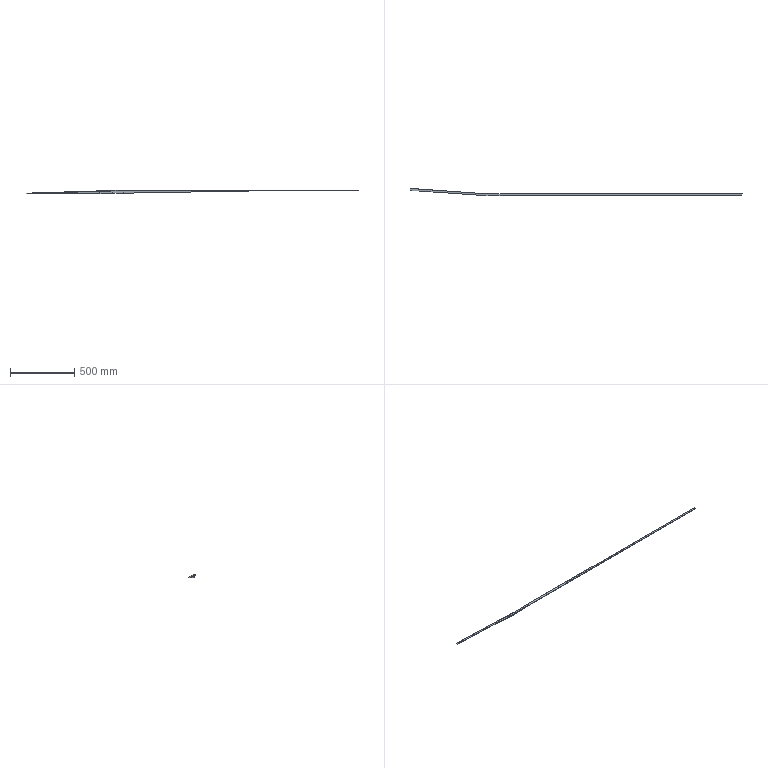Part | SolidWorks | features BaseBody 1 | 1 solid | 24 faces | box 2576 x 55.445 x 25.01 mm | volume 179602 mm3 | plane 24
STEP:
#1=CARTESIAN_POINT('',(1223.741,60.698,-2.475));
#2=VERTEX_POINT('',#1);
#3=CARTESIAN_POINT('',(180.528,60.974,-20.535));
#4=VERTEX_POINT('',#3);
#5=CARTESIAN_POINT('',(1223.741,60.698,-2.475));
#6=DIRECTION('',(-0.9999,0.0002647,-0.01731));
#7=VECTOR('',#6,1000.);
#8=LINE('',#5,#7);
#9=EDGE_CURVE('',#2,#4,#8,.T.);
#10=ORIENTED_EDGE('',*,*,#9,.F.);
#11=CARTESIAN_POINT('',(180.52,60.706,-2.934));
#12=VERTEX_POINT('',#11);
#13=CARTESIAN_POINT('',(180.52,60.706,-2.934));
#14=DIRECTION('',(1.,-0.000007674,0.0004396));
#15=VECTOR('',#14,1000.);
#16=LINE('',#13,#15);
#17=EDGE_CURVE('',#12,#2,#16,.T.);
#18=ORIENTED_EDGE('',*,*,#17,.F.);
#19=CARTESIAN_POINT('',(180.528,60.974,-20.535));
#20=DIRECTION('',(-0.0004397,-0.01523,0.9999));
#21=VECTOR('',#20,1000.);
#22=LINE('',#19,#21);
#23=EDGE_CURVE('',#4,#12,#22,.T.);
#24=ORIENTED_EDGE('',*,*,#23,.F.);
#25=EDGE_LOOP('',(#10,#18,#24));
#26=FACE_OUTER_BOUND('',#25,.T.);
#27=CARTESIAN_POINT('',(174.261,60.976,-20.643));
#28=DIRECTION('',(0.000000977,0.9999,0.01523));
#29=DIRECTION('',(0.,-0.01523,0.9999));
#30=AXIS2_PLACEMENT_3D('',#27,#28,#29);
#31=PLANE('',#30);
#32=ADVANCED_FACE('',(#26),#31,.F.);
#33=CARTESIAN_POINT('',(97.321,60.705,-2.934));
#34=VERTEX_POINT('',#33);
#35=CARTESIAN_POINT('',(180.52,60.706,-2.934));
#36=DIRECTION('',(-1.,-0.00001057,-0.000006272));
#37=VECTOR('',#36,1000.);
#38=LINE('',#35,#37);
#39=EDGE_CURVE('',#12,#34,#38,.T.);
#40=ORIENTED_EDGE('',*,*,#39,.T.);
#41=CARTESIAN_POINT('',(97.601,60.973,-20.536));
#42=VERTEX_POINT('',#41);
#43=CARTESIAN_POINT('',(97.321,60.705,-2.934));
#44=DIRECTION('',(0.01588,0.01523,-0.9998));
#45=VECTOR('',#44,1000.);
#46=LINE('',#43,#45);
#47=EDGE_CURVE('',#34,#42,#46,.T.);
#48=ORIENTED_EDGE('',*,*,#47,.T.);
#49=CARTESIAN_POINT('',(97.601,60.973,-20.536));
#50=DIRECTION('',(1.,0.00001057,0.000006272));
#51=VECTOR('',#50,1000.);
#52=LINE('',#49,#51);
#53=EDGE_CURVE('',#42,#4,#52,.T.);
#54=ORIENTED_EDGE('',*,*,#53,.T.);
#55=ORIENTED_EDGE('',*,*,#23,.T.);
#56=EDGE_LOOP('',(#40,#48,#54,#55));
#57=FACE_OUTER_BOUND('',#56,.T.);
#58=CARTESIAN_POINT('',(96.822,60.703,-2.828));
#59=DIRECTION('',(0.00001066,-0.9999,-0.01523));
#60=DIRECTION('',(0.,0.01523,-0.9999));
#61=AXIS2_PLACEMENT_3D('',#58,#59,#60);
#62=PLANE('',#61);
#63=ADVANCED_FACE('',(#57),#62,.T.);
#64=ORIENTED_EDGE('',*,*,#9,.T.);
#65=CARTESIAN_POINT('',(180.528,64.174,-20.486));
#66=VERTEX_POINT('',#65);
#67=CARTESIAN_POINT('',(180.528,60.954,-20.535));
#68=DIRECTION('',(0.,-0.9999,-0.01523));
#69=VECTOR('',#68,1000.);
#70=LINE('',#67,#69);
#71=EDGE_CURVE('',#66,#4,#70,.T.);
#72=ORIENTED_EDGE('',*,*,#71,.F.);
#73=CARTESIAN_POINT('',(1223.741,63.897,-2.427));
#74=VERTEX_POINT('',#73);
#75=CARTESIAN_POINT('',(1223.741,63.897,-2.427));
#76=DIRECTION('',(-0.9999,0.0002647,-0.01731));
#77=VECTOR('',#76,1000.);
#78=LINE('',#75,#77);
#79=EDGE_CURVE('',#74,#66,#78,.T.);
#80=ORIENTED_EDGE('',*,*,#79,.F.);
#81=CARTESIAN_POINT('',(1223.741,63.897,-2.427));
#82=DIRECTION('',(0.,0.9999,0.01523));
#83=VECTOR('',#82,1000.);
#84=LINE('',#81,#83);
#85=EDGE_CURVE('',#2,#74,#84,.T.);
#86=ORIENTED_EDGE('',*,*,#85,.F.);
#87=EDGE_LOOP('',(#64,#72,#80,#86));
#88=FACE_OUTER_BOUND('',#87,.T.);
#89=CARTESIAN_POINT('',(174.269,60.677,-20.648));
#90=DIRECTION('',(-0.01731,-0.01523,0.9997));
#91=DIRECTION('',(0.9999,0.,0.01731));
#92=AXIS2_PLACEMENT_3D('',#89,#90,#91);
#93=PLANE('',#92);
#94=ADVANCED_FACE('',(#88),#93,.F.);
#95=ORIENTED_EDGE('',*,*,#17,.T.);
#96=ORIENTED_EDGE('',*,*,#85,.T.);
#97=CARTESIAN_POINT('',(2000.001,63.891,-2.085));
#98=VERTEX_POINT('',#97);
#99=CARTESIAN_POINT('',(2000.001,63.891,-2.085));
#100=DIRECTION('',(-1.,0.000007674,-0.0004396));
#101=VECTOR('',#100,1000.);
#102=LINE('',#99,#101);
#103=EDGE_CURVE('',#98,#74,#102,.T.);
#104=ORIENTED_EDGE('',*,*,#103,.F.);
#105=CARTESIAN_POINT('',(2000.001,48.891,-2.314));
#106=VERTEX_POINT('',#105);
#107=CARTESIAN_POINT('',(2000.001,48.891,-2.314));
#108=DIRECTION('',(0.000000977,0.9999,0.01523));
#109=VECTOR('',#108,1000.);
#110=LINE('',#107,#109);
#111=EDGE_CURVE('',#106,#98,#110,.T.);
#112=ORIENTED_EDGE('',*,*,#111,.F.);
#113=CARTESIAN_POINT('',(180.52,48.905,-3.114));
#114=VERTEX_POINT('',#113);
#115=CARTESIAN_POINT('',(180.52,48.905,-3.114));
#116=DIRECTION('',(1.,-0.000007674,0.0004396));
#117=VECTOR('',#116,1000.);
#118=LINE('',#115,#117);
#119=EDGE_CURVE('',#114,#106,#118,.T.);
#120=ORIENTED_EDGE('',*,*,#119,.F.);
#121=CARTESIAN_POINT('',(180.52,48.833,-3.115));
#122=DIRECTION('',(0.,-0.9999,-0.01523));
#123=VECTOR('',#122,1000.);
#124=LINE('',#121,#123);
#125=EDGE_CURVE('',#12,#114,#124,.T.);
#126=ORIENTED_EDGE('',*,*,#125,.F.);
#127=EDGE_LOOP('',(#95,#96,#104,#112,#120,#126));
#128=FACE_OUTER_BOUND('',#127,.T.);
#129=CARTESIAN_POINT('',(180.52,63.904,-2.885));
#130=DIRECTION('',(-0.0004397,-0.01523,0.9999));
#131=DIRECTION('',(0.,-0.9999,-0.01523));
#132=AXIS2_PLACEMENT_3D('',#129,#130,#131);
#133=PLANE('',#132);
#134=ADVANCED_FACE('',(#128),#133,.F.);
#135=CARTESIAN_POINT('',(-2.947,60.757,-6.119));
#136=VERTEX_POINT('',#135);
#137=CARTESIAN_POINT('',(-2.947,60.757,-6.119));
#138=DIRECTION('',(0.9995,-0.0005189,0.03175));
#139=VECTOR('',#138,1000.);
#140=LINE('',#137,#139);
#141=EDGE_CURVE('',#136,#34,#140,.T.);
#142=ORIENTED_EDGE('',*,*,#141,.F.);
#143=CARTESIAN_POINT('',(-2.388,61.025,-23.712));
#144=VERTEX_POINT('',#143);
#145=CARTESIAN_POINT('',(-2.388,61.025,-23.712));
#146=DIRECTION('',(-0.03175,-0.01522,0.9994));
#147=VECTOR('',#146,1000.);
#148=LINE('',#145,#147);
#149=EDGE_CURVE('',#144,#136,#148,.T.);
#150=ORIENTED_EDGE('',*,*,#149,.F.);
#151=CARTESIAN_POINT('',(97.601,60.973,-20.536));
#152=DIRECTION('',(-0.9995,0.0005189,-0.03175));
#153=VECTOR('',#152,1000.);
#154=LINE('',#151,#153);
#155=EDGE_CURVE('',#42,#144,#154,.T.);
#156=ORIENTED_EDGE('',*,*,#155,.F.);
#157=ORIENTED_EDGE('',*,*,#47,.F.);
#158=EDGE_LOOP('',(#142,#150,#156,#157));
#159=FACE_OUTER_BOUND('',#158,.T.);
#160=CARTESIAN_POINT('',(-3.55,61.027,-23.836));
#161=DIRECTION('',(0.00003526,0.9999,0.01523));
#162=DIRECTION('',(0.,-0.01523,0.9999));
#163=AXIS2_PLACEMENT_3D('',#160,#161,#162);
#164=PLANE('',#163);
#165=ADVANCED_FACE('',(#159),#164,.F.);
#166=CARTESIAN_POINT('',(97.321,48.904,-3.114));
#167=VERTEX_POINT('',#166);
#168=CARTESIAN_POINT('',(180.52,48.905,-3.114));
#169=DIRECTION('',(-1.,-0.00001057,-0.000006272));
#170=VECTOR('',#169,1000.);
#171=LINE('',#168,#170);
#172=EDGE_CURVE('',#114,#167,#171,.T.);
#173=ORIENTED_EDGE('',*,*,#172,.T.);
#174=CARTESIAN_POINT('',(97.321,48.904,-3.114));
#175=DIRECTION('',(0.00001231,0.9999,0.01523));
#176=VECTOR('',#175,1000.);
#177=LINE('',#174,#176);
#178=EDGE_CURVE('',#167,#34,#177,.T.);
#179=ORIENTED_EDGE('',*,*,#178,.T.);
#180=ORIENTED_EDGE('',*,*,#39,.F.);
#181=ORIENTED_EDGE('',*,*,#125,.T.);
#182=EDGE_LOOP('',(#173,#179,#180,#181));
#183=FACE_OUTER_BOUND('',#182,.T.);
#184=CARTESIAN_POINT('',(96.822,48.833,-3.115));
#185=DIRECTION('',(0.00000611,0.01523,-0.9999));
#186=DIRECTION('',(0.,0.9999,0.01523));
#187=AXIS2_PLACEMENT_3D('',#184,#185,#186);
#188=PLANE('',#187);
#189=ADVANCED_FACE('',(#183),#188,.T.);
#190=ORIENTED_EDGE('',*,*,#53,.F.);
#191=CARTESIAN_POINT('',(97.601,64.173,-20.487));
#192=VERTEX_POINT('',#191);
#193=CARTESIAN_POINT('',(97.601,60.973,-20.536));
#194=DIRECTION('',(0.00001231,0.9999,0.01523));
#195=VECTOR('',#194,1000.);
#196=LINE('',#193,#195);
#197=EDGE_CURVE('',#42,#192,#196,.T.);
#198=ORIENTED_EDGE('',*,*,#197,.T.);
#199=CARTESIAN_POINT('',(97.601,64.173,-20.487));
#200=DIRECTION('',(1.,0.00001057,0.000006272));
#201=VECTOR('',#200,1000.);
#202=LINE('',#199,#201);
#203=EDGE_CURVE('',#192,#66,#202,.T.);
#204=ORIENTED_EDGE('',*,*,#203,.T.);
#205=ORIENTED_EDGE('',*,*,#71,.T.);
#206=EDGE_LOOP('',(#190,#198,#204,#205));
#207=FACE_OUTER_BOUND('',#206,.T.);
#208=CARTESIAN_POINT('',(97.103,60.954,-20.536));
#209=DIRECTION('',(0.00000611,0.01523,-0.9999));
#210=DIRECTION('',(0.,0.9999,0.01523));
#211=AXIS2_PLACEMENT_3D('',#208,#209,#210);
#212=PLANE('',#211);
#213=ADVANCED_FACE('',(#207),#212,.T.);
#214=ORIENTED_EDGE('',*,*,#79,.T.);
#215=CARTESIAN_POINT('',(180.519,63.857,0.3145));
#216=VERTEX_POINT('',#215);
#217=CARTESIAN_POINT('',(180.519,63.857,0.3145));
#218=DIRECTION('',(0.0004397,0.01523,-0.9999));
#219=VECTOR('',#218,1000.);
#220=LINE('',#217,#219);
#221=EDGE_CURVE('',#216,#66,#220,.T.);
#222=ORIENTED_EDGE('',*,*,#221,.F.);
#223=CARTESIAN_POINT('',(2000.,63.843,1.114));
#224=VERTEX_POINT('',#223);
#225=CARTESIAN_POINT('',(2000.,63.843,1.114));
#226=DIRECTION('',(-1.,0.000007674,-0.0004396));
#227=VECTOR('',#226,1000.);
#228=LINE('',#225,#227);
#229=EDGE_CURVE('',#224,#216,#228,.T.);
#230=ORIENTED_EDGE('',*,*,#229,.F.);
#231=CARTESIAN_POINT('',(2000.001,63.891,-2.085));
#232=DIRECTION('',(-0.0004397,-0.01523,0.9999));
#233=VECTOR('',#232,1000.);
#234=LINE('',#231,#233);
#235=EDGE_CURVE('',#98,#224,#234,.T.);
#236=ORIENTED_EDGE('',*,*,#235,.F.);
#237=ORIENTED_EDGE('',*,*,#103,.T.);
#238=EDGE_LOOP('',(#214,#222,#230,#236,#237));
#239=FACE_OUTER_BOUND('',#238,.T.);
#240=CARTESIAN_POINT('',(180.519,63.844,1.114));
#241=DIRECTION('',(-0.000000977,-0.9999,-0.01523));
#242=DIRECTION('',(0.,0.01523,-0.9999));
#243=AXIS2_PLACEMENT_3D('',#240,#241,#242);
#244=PLANE('',#243);
#245=ADVANCED_FACE('',(#239),#244,.F.);
#246=CARTESIAN_POINT('',(2000.,48.842,0.8859));
#247=VERTEX_POINT('',#246);
#248=CARTESIAN_POINT('',(2000.,63.843,1.114));
#249=DIRECTION('',(-0.000000977,-0.9999,-0.01523));
#250=VECTOR('',#249,1000.);
#251=LINE('',#248,#250);
#252=EDGE_CURVE('',#224,#247,#251,.T.);
#253=ORIENTED_EDGE('',*,*,#252,.T.);
#254=CARTESIAN_POINT('',(2000.,48.842,0.8859));
#255=DIRECTION('',(0.0004397,0.01523,-0.9999));
#256=VECTOR('',#255,1000.);
#257=LINE('',#254,#256);
#258=EDGE_CURVE('',#247,#106,#257,.T.);
#259=ORIENTED_EDGE('',*,*,#258,.T.);
#260=ORIENTED_EDGE('',*,*,#111,.T.);
#261=ORIENTED_EDGE('',*,*,#235,.T.);
#262=EDGE_LOOP('',(#253,#259,#260,#261));
#263=FACE_OUTER_BOUND('',#262,.T.);
#264=CARTESIAN_POINT('',(2000.,48.752,1.135));
#265=DIRECTION('',(1.,-0.000007674,0.0004396));
#266=DIRECTION('',(0.0004396,0.,-1.));
#267=AXIS2_PLACEMENT_3D('',#264,#265,#266);
#268=PLANE('',#267);
#269=ADVANCED_FACE('',(#263),#268,.T.);
#270=ORIENTED_EDGE('',*,*,#119,.T.);
#271=ORIENTED_EDGE('',*,*,#258,.F.);
#272=CARTESIAN_POINT('',(180.519,48.856,0.08599));
#273=VERTEX_POINT('',#272);
#274=CARTESIAN_POINT('',(180.519,48.856,0.08599));
#275=DIRECTION('',(1.,-0.000007674,0.0004396));
#276=VECTOR('',#275,1000.);
#277=LINE('',#274,#276);
#278=EDGE_CURVE('',#273,#247,#277,.T.);
#279=ORIENTED_EDGE('',*,*,#278,.F.);
#280=CARTESIAN_POINT('',(180.52,48.905,-3.114));
#281=DIRECTION('',(-0.0004396,-0.01523,0.9999));
#282=VECTOR('',#281,1000.);
#283=LINE('',#280,#282);
#284=EDGE_CURVE('',#114,#273,#283,.T.);
#285=ORIENTED_EDGE('',*,*,#284,.F.);
#286=EDGE_LOOP('',(#270,#271,#279,#285));
#287=FACE_OUTER_BOUND('',#286,.T.);
#288=CARTESIAN_POINT('',(169.602,48.905,-3.138));
#289=DIRECTION('',(0.000000977,0.9999,0.01523));
#290=DIRECTION('',(0.,-0.01523,0.9999));
#291=AXIS2_PLACEMENT_3D('',#288,#289,#290);
#292=PLANE('',#291);
#293=ADVANCED_FACE('',(#287),#292,.F.);
#294=CARTESIAN_POINT('',(-3.359,48.956,-6.312));
#295=VERTEX_POINT('',#294);
#296=CARTESIAN_POINT('',(-576.157,89.323,-23.896));
#297=VERTEX_POINT('',#296);
#298=CARTESIAN_POINT('',(-3.359,48.956,-6.312));
#299=DIRECTION('',(-0.9971,0.07027,-0.03061));
#300=VECTOR('',#299,1000.);
#301=LINE('',#298,#300);
#302=EDGE_CURVE('',#295,#297,#301,.T.);
#303=ORIENTED_EDGE('',*,*,#302,.T.);
#304=CARTESIAN_POINT('',(-575.334,101.095,-23.69));
#305=VERTEX_POINT('',#304);
#306=CARTESIAN_POINT('',(-576.157,89.323,-23.896));
#307=DIRECTION('',(0.06976,0.9974,0.01741));
#308=VECTOR('',#307,1000.);
#309=LINE('',#306,#308);
#310=EDGE_CURVE('',#297,#305,#309,.T.);
#311=ORIENTED_EDGE('',*,*,#310,.T.);
#312=CARTESIAN_POINT('',(-575.334,101.095,-23.69));
#313=DIRECTION('',(0.9971,-0.07027,0.03061));
#314=VECTOR('',#313,1000.);
#315=LINE('',#312,#314);
#316=EDGE_CURVE('',#305,#136,#315,.T.);
#317=ORIENTED_EDGE('',*,*,#316,.T.);
#318=ORIENTED_EDGE('',*,*,#141,.T.);
#319=ORIENTED_EDGE('',*,*,#178,.F.);
#320=CARTESIAN_POINT('',(97.321,48.904,-3.114));
#321=DIRECTION('',(-0.9995,0.0005189,-0.03175));
#322=VECTOR('',#321,1000.);
#323=LINE('',#320,#322);
#324=EDGE_CURVE('',#167,#295,#323,.T.);
#325=ORIENTED_EDGE('',*,*,#324,.T.);
#326=EDGE_LOOP('',(#303,#311,#317,#318,#319,#325));
#327=FACE_OUTER_BOUND('',#326,.T.);
#328=CARTESIAN_POINT('',(97.327,48.904,-3.114));
#329=DIRECTION('',(0.03175,0.01522,-0.9994));
#330=DIRECTION('',(-0.9995,0.,-0.03176));
#331=AXIS2_PLACEMENT_3D('',#328,#329,#330);
#332=PLANE('',#331);
#333=ADVANCED_FACE('',(#327),#332,.T.);
#334=ORIENTED_EDGE('',*,*,#149,.T.);
#335=ORIENTED_EDGE('',*,*,#316,.F.);
#336=CARTESIAN_POINT('',(-575.334,101.095,-23.69));
#337=DIRECTION('',(0.9976,-0.06977,-0.00003666));
#338=VECTOR('',#337,1000.);
#339=LINE('',#336,#338);
#340=EDGE_CURVE('',#305,#144,#339,.T.);
#341=ORIENTED_EDGE('',*,*,#340,.T.);
#342=EDGE_LOOP('',(#334,#335,#341));
#343=FACE_OUTER_BOUND('',#342,.T.);
#344=CARTESIAN_POINT('',(-578.772,101.338,-23.817));
#345=DIRECTION('',(-0.06976,-0.9974,-0.01741));
#346=DIRECTION('',(0.9976,-0.06977,0.));
#347=AXIS2_PLACEMENT_3D('',#344,#345,#346);
#348=PLANE('',#347);
#349=ADVANCED_FACE('',(#343),#348,.T.);
#350=ORIENTED_EDGE('',*,*,#197,.F.);
#351=ORIENTED_EDGE('',*,*,#155,.T.);
#352=CARTESIAN_POINT('',(-2.164,64.224,-23.656));
#353=VERTEX_POINT('',#352);
#354=CARTESIAN_POINT('',(-2.388,61.025,-23.712));
#355=DIRECTION('',(0.06976,0.9974,0.01741));
#356=VECTOR('',#355,1000.);
#357=LINE('',#354,#356);
#358=EDGE_CURVE('',#144,#353,#357,.T.);
#359=ORIENTED_EDGE('',*,*,#358,.T.);
#360=CARTESIAN_POINT('',(-2.164,64.224,-23.656));
#361=DIRECTION('',(0.9995,-0.0005189,0.03175));
#362=VECTOR('',#361,1000.);
#363=LINE('',#360,#362);
#364=EDGE_CURVE('',#353,#192,#363,.T.);
#365=ORIENTED_EDGE('',*,*,#364,.T.);
#366=EDGE_LOOP('',(#350,#351,#359,#365));
#367=FACE_OUTER_BOUND('',#366,.T.);
#368=CARTESIAN_POINT('',(98.203,60.954,-20.517));
#369=DIRECTION('',(0.03175,0.01522,-0.9994));
#370=DIRECTION('',(-0.9995,0.,-0.03176));
#371=AXIS2_PLACEMENT_3D('',#368,#369,#370);
#372=PLANE('',#371);
#373=ADVANCED_FACE('',(#367),#372,.T.);
#374=CARTESIAN_POINT('',(97.27,48.855,0.08547));
#375=VERTEX_POINT('',#374);
#376=CARTESIAN_POINT('',(180.519,48.856,0.08599));
#377=DIRECTION('',(-1.,-0.00001057,-0.000006272));
#378=VECTOR('',#377,1000.);
#379=LINE('',#376,#378);
#380=EDGE_CURVE('',#273,#375,#379,.T.);
#381=ORIENTED_EDGE('',*,*,#380,.T.);
#382=CARTESIAN_POINT('',(97.27,48.855,0.08547));
#383=DIRECTION('',(0.01588,0.01523,-0.9998));
#384=VECTOR('',#383,1000.);
#385=LINE('',#382,#384);
#386=EDGE_CURVE('',#375,#167,#385,.T.);
#387=ORIENTED_EDGE('',*,*,#386,.T.);
#388=ORIENTED_EDGE('',*,*,#172,.F.);
#389=ORIENTED_EDGE('',*,*,#284,.T.);
#390=EDGE_LOOP('',(#381,#387,#388,#389));
#391=FACE_OUTER_BOUND('',#390,.T.);
#392=CARTESIAN_POINT('',(96.771,48.855,0.1052));
#393=DIRECTION('',(0.00001066,-0.9999,-0.01523));
#394=DIRECTION('',(0.,0.01523,-0.9999));
#395=AXIS2_PLACEMENT_3D('',#392,#393,#394);
#396=PLANE('',#395);
#397=ADVANCED_FACE('',(#391),#396,.T.);
#398=ORIENTED_EDGE('',*,*,#203,.F.);
#399=CARTESIAN_POINT('',(97.271,63.856,0.314));
#400=VERTEX_POINT('',#399);
#401=CARTESIAN_POINT('',(97.601,64.173,-20.487));
#402=DIRECTION('',(-0.01588,-0.01523,0.9998));
#403=VECTOR('',#402,1000.);
#404=LINE('',#401,#403);
#405=EDGE_CURVE('',#192,#400,#404,.T.);
#406=ORIENTED_EDGE('',*,*,#405,.T.);
#407=CARTESIAN_POINT('',(97.271,63.856,0.314));
#408=DIRECTION('',(1.,0.00001057,0.000006272));
#409=VECTOR('',#408,1000.);
#410=LINE('',#407,#409);
#411=EDGE_CURVE('',#400,#216,#410,.T.);
#412=ORIENTED_EDGE('',*,*,#411,.T.);
#413=ORIENTED_EDGE('',*,*,#221,.T.);
#414=EDGE_LOOP('',(#398,#406,#412,#413));
#415=FACE_OUTER_BOUND('',#414,.T.);
#416=CARTESIAN_POINT('',(96.771,64.175,-20.612));
#417=DIRECTION('',(-0.00001066,0.9999,0.01523));
#418=DIRECTION('',(0.,-0.01523,0.9999));
#419=AXIS2_PLACEMENT_3D('',#416,#417,#418);
#420=PLANE('',#419);
#421=ADVANCED_FACE('',(#415),#420,.T.);
#422=ORIENTED_EDGE('',*,*,#278,.T.);
#423=ORIENTED_EDGE('',*,*,#252,.F.);
#424=ORIENTED_EDGE('',*,*,#229,.T.);
#425=CARTESIAN_POINT('',(180.519,63.947,0.3159));
#426=DIRECTION('',(0.,0.9999,0.01523));
#427=VECTOR('',#426,1000.);
#428=LINE('',#425,#427);
#429=EDGE_CURVE('',#273,#216,#428,.T.);
#430=ORIENTED_EDGE('',*,*,#429,.F.);
#431=EDGE_LOOP('',(#422,#423,#424,#430));
#432=FACE_OUTER_BOUND('',#431,.T.);
#433=CARTESIAN_POINT('',(169.602,48.764,0.07979));
#434=DIRECTION('',(0.0004397,0.01523,-0.9999));
#435=DIRECTION('',(0.,0.9999,0.01523));
#436=AXIS2_PLACEMENT_3D('',#433,#434,#435);
#437=PLANE('',#436);
#438=ADVANCED_FACE('',(#432),#437,.F.);
#439=CARTESIAN_POINT('',(-576.259,89.275,-20.698));
#440=VERTEX_POINT('',#439);
#441=CARTESIAN_POINT('',(-575.213,104.238,-20.437));
#442=VERTEX_POINT('',#441);
#443=CARTESIAN_POINT('',(-576.259,89.275,-20.698));
#444=DIRECTION('',(0.06976,0.9974,0.01741));
#445=VECTOR('',#444,1000.);
#446=LINE('',#443,#445);
#447=EDGE_CURVE('',#440,#442,#446,.T.);
#448=ORIENTED_EDGE('',*,*,#447,.T.);
#449=CARTESIAN_POINT('',(-575.111,104.287,-23.635));
#450=VERTEX_POINT('',#449);
#451=CARTESIAN_POINT('',(-575.213,104.238,-20.437));
#452=DIRECTION('',(0.03175,0.01522,-0.9994));
#453=VECTOR('',#452,1000.);
#454=LINE('',#451,#453);
#455=EDGE_CURVE('',#442,#450,#454,.T.);
#456=ORIENTED_EDGE('',*,*,#455,.T.);
#457=CARTESIAN_POINT('',(-575.111,104.287,-23.635));
#458=DIRECTION('',(-0.06976,-0.9974,-0.01741));
#459=VECTOR('',#458,1000.);
#460=LINE('',#457,#459);
#461=EDGE_CURVE('',#450,#305,#460,.T.);
#462=ORIENTED_EDGE('',*,*,#461,.T.);
#463=ORIENTED_EDGE('',*,*,#310,.F.);
#464=CARTESIAN_POINT('',(-576.157,89.323,-23.896));
#465=DIRECTION('',(-0.03175,-0.01522,0.9994));
#466=VECTOR('',#465,1000.);
#467=LINE('',#464,#466);
#468=EDGE_CURVE('',#297,#440,#467,.T.);
#469=ORIENTED_EDGE('',*,*,#468,.T.);
#470=EDGE_LOOP('',(#448,#456,#462,#463,#469));
#471=FACE_OUTER_BOUND('',#470,.T.);
#472=CARTESIAN_POINT('',(-575.103,104.286,-23.896));
#473=DIRECTION('',(-0.9971,0.07027,-0.03061));
#474=DIRECTION('',(-0.0703,-0.9975,0.));
#475=AXIS2_PLACEMENT_3D('',#472,#473,#474);
#476=PLANE('',#475);
#477=ADVANCED_FACE('',(#471),#476,.T.);
#478=CARTESIAN_POINT('',(-3.461,48.908,-3.114));
#479=VERTEX_POINT('',#478);
#480=CARTESIAN_POINT('',(-3.461,48.908,-3.114));
#481=DIRECTION('',(-0.9971,0.07027,-0.03061));
#482=VECTOR('',#481,1000.);
#483=LINE('',#480,#482);
#484=EDGE_CURVE('',#479,#440,#483,.T.);
#485=ORIENTED_EDGE('',*,*,#484,.T.);
#486=ORIENTED_EDGE('',*,*,#468,.F.);
#487=ORIENTED_EDGE('',*,*,#302,.F.);
#488=CARTESIAN_POINT('',(-3.359,48.956,-6.312));
#489=DIRECTION('',(-0.03175,-0.01522,0.9994));
#490=VECTOR('',#489,1000.);
#491=LINE('',#488,#490);
#492=EDGE_CURVE('',#295,#479,#491,.T.);
#493=ORIENTED_EDGE('',*,*,#492,.T.);
#494=EDGE_LOOP('',(#485,#486,#487,#493));
#495=FACE_OUTER_BOUND('',#494,.T.);
#496=CARTESIAN_POINT('',(-579.692,89.573,-24.021));
#497=DIRECTION('',(-0.06976,-0.9974,-0.01741));
#498=DIRECTION('',(0.9976,-0.06977,0.));
#499=AXIS2_PLACEMENT_3D('',#496,#497,#498);
#500=PLANE('',#499);
#501=ADVANCED_FACE('',(#495),#500,.T.);
#502=CARTESIAN_POINT('',(-3.461,48.908,-3.114));
#503=DIRECTION('',(0.9995,-0.0005189,0.03175));
#504=VECTOR('',#503,1000.);
#505=LINE('',#502,#504);
#506=EDGE_CURVE('',#479,#375,#505,.T.);
#507=ORIENTED_EDGE('',*,*,#506,.F.);
#508=ORIENTED_EDGE('',*,*,#492,.F.);
#509=ORIENTED_EDGE('',*,*,#324,.F.);
#510=ORIENTED_EDGE('',*,*,#386,.F.);
#511=EDGE_LOOP('',(#507,#508,#509,#510));
#512=FACE_OUTER_BOUND('',#511,.T.);
#513=CARTESIAN_POINT('',(-4.066,48.957,-6.351));
#514=DIRECTION('',(0.00003526,0.9999,0.01523));
#515=DIRECTION('',(0.,-0.01523,0.9999));
#516=AXIS2_PLACEMENT_3D('',#513,#514,#515);
#517=PLANE('',#516);
#518=ADVANCED_FACE('',(#512),#517,.F.);
#519=ORIENTED_EDGE('',*,*,#340,.F.);
#520=ORIENTED_EDGE('',*,*,#461,.F.);
#521=CARTESIAN_POINT('',(-2.276,64.224,-23.656));
#522=VERTEX_POINT('',#521);
#523=CARTESIAN_POINT('',(-2.276,64.224,-23.656));
#524=DIRECTION('',(-0.9976,0.06977,0.00003666));
#525=VECTOR('',#524,1000.);
#526=LINE('',#523,#525);
#527=EDGE_CURVE('',#522,#450,#526,.T.);
#528=ORIENTED_EDGE('',*,*,#527,.F.);
#529=CARTESIAN_POINT('',(-288.749,64.23,-23.993));
#530=DIRECTION('',(-1.,0.00002046,-0.001178));
#531=VECTOR('',#530,1000.);
#532=LINE('',#529,#531);
#533=EDGE_CURVE('',#353,#522,#532,.T.);
#534=ORIENTED_EDGE('',*,*,#533,.F.);
#535=ORIENTED_EDGE('',*,*,#358,.F.);
#536=EDGE_LOOP('',(#519,#520,#528,#534,#535));
#537=FACE_OUTER_BOUND('',#536,.T.);
#538=CARTESIAN_POINT('',(-575.334,104.287,-23.635));
#539=DIRECTION('',(-0.001178,-0.01737,0.9998));
#540=DIRECTION('',(0.,-0.9998,-0.01737));
#541=AXIS2_PLACEMENT_3D('',#538,#539,#540);
#542=PLANE('',#541);
#543=ADVANCED_FACE('',(#537),#542,.F.);
#544=ORIENTED_EDGE('',*,*,#533,.T.);
#545=CARTESIAN_POINT('',(-2.937,63.908,-2.869));
#546=VERTEX_POINT('',#545);
#547=CARTESIAN_POINT('',(-2.937,63.908,-2.869));
#548=DIRECTION('',(0.03175,0.01522,-0.9994));
#549=VECTOR('',#548,1000.);
#550=LINE('',#547,#549);
#551=EDGE_CURVE('',#546,#522,#550,.T.);
#552=ORIENTED_EDGE('',*,*,#551,.F.);
#553=CARTESIAN_POINT('',(97.271,63.856,0.314));
#554=DIRECTION('',(-0.9995,0.0005189,-0.03175));
#555=VECTOR('',#554,1000.);
#556=LINE('',#553,#555);
#557=EDGE_CURVE('',#400,#546,#556,.T.);
#558=ORIENTED_EDGE('',*,*,#557,.F.);
#559=ORIENTED_EDGE('',*,*,#405,.F.);
#560=ORIENTED_EDGE('',*,*,#364,.F.);
#561=EDGE_LOOP('',(#544,#552,#558,#559,#560));
#562=FACE_OUTER_BOUND('',#561,.T.);
#563=CARTESIAN_POINT('',(-2.937,63.859,0.314));
#564=DIRECTION('',(-0.00003526,-0.9999,-0.01523));
#565=DIRECTION('',(0.,0.01523,-0.9999));
#566=AXIS2_PLACEMENT_3D('',#563,#564,#565);
#567=PLANE('',#566);
#568=ADVANCED_FACE('',(#562),#567,.F.);
#569=ORIENTED_EDGE('',*,*,#411,.F.);
#570=CARTESIAN_POINT('',(97.271,63.856,0.314));
#571=DIRECTION('',(-0.0000123,-0.9999,-0.01523));
#572=VECTOR('',#571,1000.);
#573=LINE('',#570,#572);
#574=EDGE_CURVE('',#400,#375,#573,.T.);
#575=ORIENTED_EDGE('',*,*,#574,.T.);
#576=ORIENTED_EDGE('',*,*,#380,.F.);
#577=ORIENTED_EDGE('',*,*,#429,.T.);
#578=EDGE_LOOP('',(#569,#575,#576,#577));
#579=FACE_OUTER_BOUND('',#578,.T.);
#580=CARTESIAN_POINT('',(96.771,63.947,0.3154));
#581=DIRECTION('',(-0.00000611,-0.01523,0.9999));
#582=DIRECTION('',(0.,-0.9999,-0.01523));
#583=AXIS2_PLACEMENT_3D('',#580,#581,#582);
#584=PLANE('',#583);
#585=ADVANCED_FACE('',(#579),#584,.T.);
#586=CARTESIAN_POINT('',(-575.213,104.238,-20.437));
#587=DIRECTION('',(0.9971,-0.07027,0.03061));
#588=VECTOR('',#587,1000.);
#589=LINE('',#586,#588);
#590=EDGE_CURVE('',#442,#546,#589,.T.);
#591=ORIENTED_EDGE('',*,*,#590,.T.);
#592=ORIENTED_EDGE('',*,*,#551,.T.);
#593=ORIENTED_EDGE('',*,*,#527,.T.);
#594=ORIENTED_EDGE('',*,*,#455,.F.);
#595=EDGE_LOOP('',(#591,#592,#593,#594));
#596=FACE_OUTER_BOUND('',#595,.T.);
#597=CARTESIAN_POINT('',(1.161,63.986,-23.781));
#598=DIRECTION('',(0.06976,0.9974,0.01741));
#599=DIRECTION('',(-0.9976,0.06977,0.));
#600=AXIS2_PLACEMENT_3D('',#597,#598,#599);
#601=PLANE('',#600);
#602=ADVANCED_FACE('',(#596),#601,.T.);
#603=ORIENTED_EDGE('',*,*,#590,.F.);
#604=ORIENTED_EDGE('',*,*,#447,.F.);
#605=ORIENTED_EDGE('',*,*,#484,.F.);
#606=ORIENTED_EDGE('',*,*,#506,.T.);
#607=ORIENTED_EDGE('',*,*,#574,.F.);
#608=ORIENTED_EDGE('',*,*,#557,.T.);
#609=EDGE_LOOP('',(#603,#604,#605,#606,#607,#608));
#610=FACE_OUTER_BOUND('',#609,.T.);
#611=CARTESIAN_POINT('',(-576.239,48.855,-21.313));
#612=DIRECTION('',(-0.03175,-0.01522,0.9994));
#613=DIRECTION('',(0.9995,0.,0.03176));
#614=AXIS2_PLACEMENT_3D('',#611,#612,#613);
#615=PLANE('',#614);
#616=ADVANCED_FACE('',(#610),#615,.T.);
#617=CLOSED_SHELL('',(#32,#63,#94,#134,#165,#189,#213,#245,#269,#293,#333,#349,#373,#397,#421,#438,#477,#501,#518,#543,#568,#585,#602,#616));
#618=MANIFOLD_SOLID_BREP('',#617);
#619=CARTESIAN_POINT('',(0.,0.,0.));
#620=DIRECTION('',(0.,0.,1.));
#621=DIRECTION('',(1.,0.,0.));
#622=AXIS2_PLACEMENT_3D('',#619,#620,#621);
#623=(LENGTH_UNIT()NAMED_UNIT(*)SI_UNIT(.MILLI.,.METRE.));
#624=UNCERTAINTY_MEASURE_WITH_UNIT(LENGTH_MEASURE(0.00001),#623,'','');
#625=(NAMED_UNIT(*)PLANE_ANGLE_UNIT()SI_UNIT($,.RADIAN.));
#626=(NAMED_UNIT(*)SI_UNIT($,.STERADIAN.)SOLID_ANGLE_UNIT());
#627=(GEOMETRIC_REPRESENTATION_CONTEXT(3)GLOBAL_UNCERTAINTY_ASSIGNED_CONTEXT((#624))GLOBAL_UNIT_ASSIGNED_CONTEXT((#623,#625,#626))REPRESENTATION_CONTEXT('',''));
#628=ADVANCED_BREP_SHAPE_REPRESENTATION('',(#618,#622),#627);